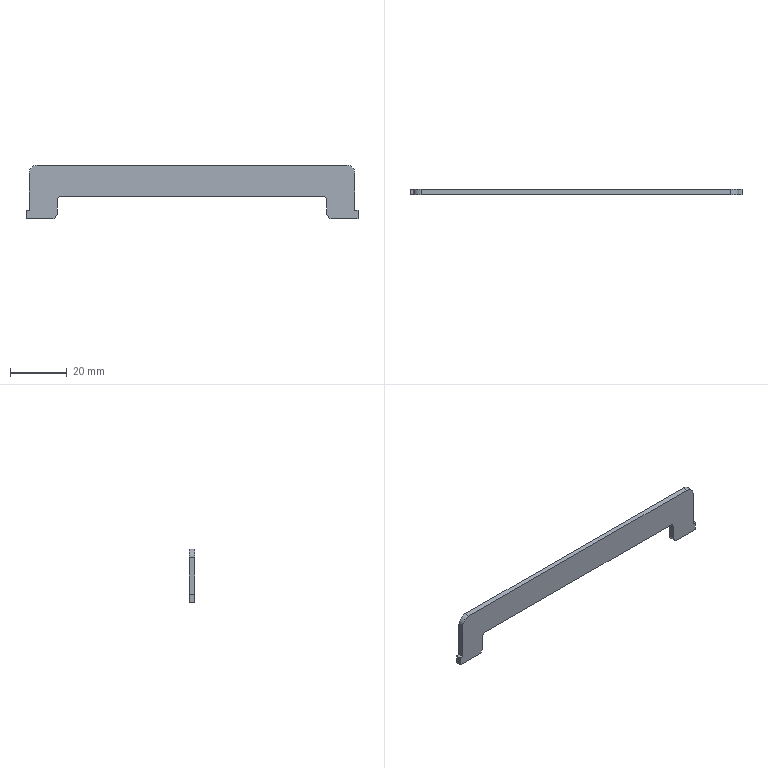Part | STEP file | 200 mesh_id2122 | 1 solid | 20 faces | box 117 x 1.9 x 19 mm | volume 2704 mm3 | plane 14 | cylinder 6 | commonest cylinder face diameters 3 x2 4 x2 6 x2
STEP:
#1=CARTESIAN_POINT('',(-16913.748,-3988.719,48.1));
#2=VERTEX_POINT('',#1);
#3=CARTESIAN_POINT('',(-17022.548,-3988.719,48.1));
#4=VERTEX_POINT('',#3);
#5=CARTESIAN_POINT('',(-16912.148,-3988.719,48.1));
#6=DIRECTION('',(-1.,0.,0.));
#7=VECTOR('',#6,1.);
#8=LINE('',#5,#7);
#9=EDGE_CURVE('',#2,#4,#8,.T.);
#10=ORIENTED_EDGE('',*,*,#9,.F.);
#11=CARTESIAN_POINT('',(-16913.748,-3986.819,48.1));
#12=VERTEX_POINT('',#11);
#13=CARTESIAN_POINT('',(-16913.748,-3988.744,48.1));
#14=DIRECTION('',(0.,1.,0.));
#15=VECTOR('',#14,1.);
#16=LINE('',#13,#15);
#17=EDGE_CURVE('',#2,#12,#16,.T.);
#18=ORIENTED_EDGE('',*,*,#17,.T.);
#19=CARTESIAN_POINT('',(-17022.548,-3986.819,48.1));
#20=VERTEX_POINT('',#19);
#21=CARTESIAN_POINT('',(-16912.148,-3986.819,48.1));
#22=DIRECTION('',(-1.,0.,0.));
#23=VECTOR('',#22,1.);
#24=LINE('',#21,#23);
#25=EDGE_CURVE('',#12,#20,#24,.T.);
#26=ORIENTED_EDGE('',*,*,#25,.T.);
#27=CARTESIAN_POINT('',(-17022.548,-3988.744,48.1));
#28=DIRECTION('',(0.,-1.,0.));
#29=VECTOR('',#28,1.);
#30=LINE('',#27,#29);
#31=EDGE_CURVE('',#20,#4,#30,.T.);
#32=ORIENTED_EDGE('',*,*,#31,.T.);
#33=EDGE_LOOP('',(#10,#18,#26,#32));
#34=FACE_OUTER_BOUND('',#33,.T.);
#35=CARTESIAN_POINT('',(-16912.148,-3988.744,48.1));
#36=DIRECTION('',(0.,0.,-1.));
#37=DIRECTION('',(1.,0.,0.));
#38=AXIS2_PLACEMENT_3D('',#35,#36,#37);
#39=PLANE('',#38);
#40=ADVANCED_FACE('',(#34),#39,.F.);
#41=CARTESIAN_POINT('',(-17025.548,-3988.719,45.1));
#42=VERTEX_POINT('',#41);
#43=CARTESIAN_POINT('',(-17025.548,-3988.719,32.1));
#44=VERTEX_POINT('',#43);
#45=CARTESIAN_POINT('',(-17025.548,-3988.719,46.6));
#46=DIRECTION('',(0.,0.,-1.));
#47=VECTOR('',#46,1.);
#48=LINE('',#45,#47);
#49=EDGE_CURVE('',#42,#44,#48,.T.);
#50=ORIENTED_EDGE('',*,*,#49,.F.);
#51=CARTESIAN_POINT('',(-17025.548,-3986.819,45.1));
#52=VERTEX_POINT('',#51);
#53=CARTESIAN_POINT('',(-17025.548,-3988.744,45.1));
#54=DIRECTION('',(0.,1.,0.));
#55=VECTOR('',#54,1.);
#56=LINE('',#53,#55);
#57=EDGE_CURVE('',#42,#52,#56,.T.);
#58=ORIENTED_EDGE('',*,*,#57,.T.);
#59=CARTESIAN_POINT('',(-17025.548,-3986.819,32.1));
#60=VERTEX_POINT('',#59);
#61=CARTESIAN_POINT('',(-17025.548,-3986.819,46.6));
#62=DIRECTION('',(0.,0.,-1.));
#63=VECTOR('',#62,1.);
#64=LINE('',#61,#63);
#65=EDGE_CURVE('',#52,#60,#64,.T.);
#66=ORIENTED_EDGE('',*,*,#65,.T.);
#67=CARTESIAN_POINT('',(-17025.548,-3988.744,32.1));
#68=DIRECTION('',(0.,1.,0.));
#69=VECTOR('',#68,1.);
#70=LINE('',#67,#69);
#71=EDGE_CURVE('',#44,#60,#70,.T.);
#72=ORIENTED_EDGE('',*,*,#71,.F.);
#73=EDGE_LOOP('',(#50,#58,#66,#72));
#74=FACE_OUTER_BOUND('',#73,.T.);
#75=CARTESIAN_POINT('',(-17025.548,-3988.744,46.6));
#76=DIRECTION('',(1.,0.,0.));
#77=DIRECTION('',(0.,1.,0.));
#78=AXIS2_PLACEMENT_3D('',#75,#76,#77);
#79=PLANE('',#78);
#80=ADVANCED_FACE('',(#74),#79,.F.);
#81=CARTESIAN_POINT('',(-17026.648,-3986.819,32.1));
#82=VERTEX_POINT('',#81);
#83=CARTESIAN_POINT('',(-17025.648,-3986.819,32.1));
#84=DIRECTION('',(-1.,0.,0.));
#85=VECTOR('',#84,1.);
#86=LINE('',#83,#85);
#87=EDGE_CURVE('',#60,#82,#86,.T.);
#88=ORIENTED_EDGE('',*,*,#87,.T.);
#89=CARTESIAN_POINT('',(-17026.648,-3988.719,32.1));
#90=VERTEX_POINT('',#89);
#91=CARTESIAN_POINT('',(-17026.648,-3988.744,32.1));
#92=DIRECTION('',(0.,1.,0.));
#93=VECTOR('',#92,1.);
#94=LINE('',#91,#93);
#95=EDGE_CURVE('',#90,#82,#94,.T.);
#96=ORIENTED_EDGE('',*,*,#95,.F.);
#97=CARTESIAN_POINT('',(-17025.648,-3988.719,32.1));
#98=DIRECTION('',(-1.,0.,0.));
#99=VECTOR('',#98,1.);
#100=LINE('',#97,#99);
#101=EDGE_CURVE('',#44,#90,#100,.T.);
#102=ORIENTED_EDGE('',*,*,#101,.F.);
#103=ORIENTED_EDGE('',*,*,#71,.T.);
#104=EDGE_LOOP('',(#88,#96,#102,#103));
#105=FACE_OUTER_BOUND('',#104,.T.);
#106=CARTESIAN_POINT('',(-17025.648,-3988.744,32.1));
#107=DIRECTION('',(0.,0.,-1.));
#108=DIRECTION('',(0.,1.,0.));
#109=AXIS2_PLACEMENT_3D('',#106,#107,#108);
#110=PLANE('',#109);
#111=ADVANCED_FACE('',(#105),#110,.F.);
#112=CARTESIAN_POINT('',(-17026.648,-3986.819,29.1));
#113=VERTEX_POINT('',#112);
#114=CARTESIAN_POINT('',(-17026.648,-3986.819,32.1));
#115=DIRECTION('',(0.,0.,-1.));
#116=VECTOR('',#115,1.);
#117=LINE('',#114,#116);
#118=EDGE_CURVE('',#82,#113,#117,.T.);
#119=ORIENTED_EDGE('',*,*,#118,.T.);
#120=CARTESIAN_POINT('',(-17026.648,-3988.719,29.1));
#121=VERTEX_POINT('',#120);
#122=CARTESIAN_POINT('',(-17026.648,-3988.744,29.1));
#123=DIRECTION('',(0.,1.,0.));
#124=VECTOR('',#123,1.);
#125=LINE('',#122,#124);
#126=EDGE_CURVE('',#121,#113,#125,.T.);
#127=ORIENTED_EDGE('',*,*,#126,.F.);
#128=CARTESIAN_POINT('',(-17026.648,-3988.719,32.1));
#129=DIRECTION('',(0.,0.,-1.));
#130=VECTOR('',#129,1.);
#131=LINE('',#128,#130);
#132=EDGE_CURVE('',#90,#121,#131,.T.);
#133=ORIENTED_EDGE('',*,*,#132,.F.);
#134=ORIENTED_EDGE('',*,*,#95,.T.);
#135=EDGE_LOOP('',(#119,#127,#133,#134));
#136=FACE_OUTER_BOUND('',#135,.T.);
#137=CARTESIAN_POINT('',(-17026.648,-3988.744,32.1));
#138=DIRECTION('',(1.,0.,0.));
#139=DIRECTION('',(0.,1.,0.));
#140=AXIS2_PLACEMENT_3D('',#137,#138,#139);
#141=PLANE('',#140);
#142=ADVANCED_FACE('',(#136),#141,.F.);
#143=CARTESIAN_POINT('',(-17017.648,-3986.819,29.1));
#144=VERTEX_POINT('',#143);
#145=CARTESIAN_POINT('',(-17026.648,-3986.819,29.1));
#146=DIRECTION('',(1.,0.,0.));
#147=VECTOR('',#146,1.);
#148=LINE('',#145,#147);
#149=EDGE_CURVE('',#113,#144,#148,.T.);
#150=ORIENTED_EDGE('',*,*,#149,.T.);
#151=CARTESIAN_POINT('',(-17017.648,-3988.719,29.1));
#152=VERTEX_POINT('',#151);
#153=CARTESIAN_POINT('',(-17017.648,-3988.744,29.1));
#154=DIRECTION('',(0.,-1.,0.));
#155=VECTOR('',#154,1.);
#156=LINE('',#153,#155);
#157=EDGE_CURVE('',#144,#152,#156,.T.);
#158=ORIENTED_EDGE('',*,*,#157,.T.);
#159=CARTESIAN_POINT('',(-17026.648,-3988.719,29.1));
#160=DIRECTION('',(1.,0.,0.));
#161=VECTOR('',#160,1.);
#162=LINE('',#159,#161);
#163=EDGE_CURVE('',#121,#152,#162,.T.);
#164=ORIENTED_EDGE('',*,*,#163,.F.);
#165=ORIENTED_EDGE('',*,*,#126,.T.);
#166=EDGE_LOOP('',(#150,#158,#164,#165));
#167=FACE_OUTER_BOUND('',#166,.T.);
#168=CARTESIAN_POINT('',(-17026.648,-3988.744,29.1));
#169=DIRECTION('',(0.,0.,1.));
#170=DIRECTION('',(0.,-1.,0.));
#171=AXIS2_PLACEMENT_3D('',#168,#169,#170);
#172=PLANE('',#171);
#173=ADVANCED_FACE('',(#167),#172,.F.);
#174=CARTESIAN_POINT('',(-17015.648,-3986.819,31.1));
#175=VERTEX_POINT('',#174);
#176=CARTESIAN_POINT('',(-17015.648,-3986.819,35.6));
#177=VERTEX_POINT('',#176);
#178=CARTESIAN_POINT('',(-17015.648,-3986.819,29.1));
#179=DIRECTION('',(0.,0.,1.));
#180=VECTOR('',#179,1.);
#181=LINE('',#178,#180);
#182=EDGE_CURVE('',#175,#177,#181,.T.);
#183=ORIENTED_EDGE('',*,*,#182,.T.);
#184=CARTESIAN_POINT('',(-17015.648,-3988.719,35.6));
#185=VERTEX_POINT('',#184);
#186=CARTESIAN_POINT('',(-17015.648,-3988.719,35.6));
#187=DIRECTION('',(0.,-1.,0.));
#188=VECTOR('',#187,1.);
#189=LINE('',#186,#188);
#190=EDGE_CURVE('',#177,#185,#189,.T.);
#191=ORIENTED_EDGE('',*,*,#190,.T.);
#192=CARTESIAN_POINT('',(-17015.648,-3988.719,31.1));
#193=VERTEX_POINT('',#192);
#194=CARTESIAN_POINT('',(-17015.648,-3988.719,29.1));
#195=DIRECTION('',(0.,0.,1.));
#196=VECTOR('',#195,1.);
#197=LINE('',#194,#196);
#198=EDGE_CURVE('',#193,#185,#197,.T.);
#199=ORIENTED_EDGE('',*,*,#198,.F.);
#200=CARTESIAN_POINT('',(-17015.648,-3988.744,31.1));
#201=DIRECTION('',(0.,1.,0.));
#202=VECTOR('',#201,1.);
#203=LINE('',#200,#202);
#204=EDGE_CURVE('',#193,#175,#203,.T.);
#205=ORIENTED_EDGE('',*,*,#204,.T.);
#206=EDGE_LOOP('',(#183,#191,#199,#205));
#207=FACE_OUTER_BOUND('',#206,.T.);
#208=CARTESIAN_POINT('',(-17015.648,-3988.744,29.1));
#209=DIRECTION('',(-1.,0.,0.));
#210=DIRECTION('',(0.,-1.,0.));
#211=AXIS2_PLACEMENT_3D('',#208,#209,#210);
#212=PLANE('',#211);
#213=ADVANCED_FACE('',(#207),#212,.F.);
#214=CARTESIAN_POINT('',(-17014.148,-3988.719,37.1));
#215=VERTEX_POINT('',#214);
#216=CARTESIAN_POINT('',(-16922.148,-3988.719,37.1));
#217=VERTEX_POINT('',#216);
#218=CARTESIAN_POINT('',(-17015.648,-3988.719,37.1));
#219=DIRECTION('',(1.,0.,0.));
#220=VECTOR('',#219,1.);
#221=LINE('',#218,#220);
#222=EDGE_CURVE('',#215,#217,#221,.T.);
#223=ORIENTED_EDGE('',*,*,#222,.F.);
#224=CARTESIAN_POINT('',(-17014.148,-3986.819,37.1));
#225=VERTEX_POINT('',#224);
#226=CARTESIAN_POINT('',(-17014.148,-3986.819,37.1));
#227=DIRECTION('',(0.,1.,0.));
#228=VECTOR('',#227,1.);
#229=LINE('',#226,#228);
#230=EDGE_CURVE('',#215,#225,#229,.T.);
#231=ORIENTED_EDGE('',*,*,#230,.T.);
#232=CARTESIAN_POINT('',(-16922.148,-3986.819,37.1));
#233=VERTEX_POINT('',#232);
#234=CARTESIAN_POINT('',(-17015.648,-3986.819,37.1));
#235=DIRECTION('',(1.,0.,0.));
#236=VECTOR('',#235,1.);
#237=LINE('',#234,#236);
#238=EDGE_CURVE('',#225,#233,#237,.T.);
#239=ORIENTED_EDGE('',*,*,#238,.T.);
#240=CARTESIAN_POINT('',(-16922.148,-3988.719,37.1));
#241=DIRECTION('',(0.,-1.,0.));
#242=VECTOR('',#241,1.);
#243=LINE('',#240,#242);
#244=EDGE_CURVE('',#233,#217,#243,.T.);
#245=ORIENTED_EDGE('',*,*,#244,.T.);
#246=EDGE_LOOP('',(#223,#231,#239,#245));
#247=FACE_OUTER_BOUND('',#246,.T.);
#248=CARTESIAN_POINT('',(-17015.648,-3988.744,37.1));
#249=DIRECTION('',(0.,0.,1.));
#250=DIRECTION('',(0.,-1.,0.));
#251=AXIS2_PLACEMENT_3D('',#248,#249,#250);
#252=PLANE('',#251);
#253=ADVANCED_FACE('',(#247),#252,.F.);
#254=CARTESIAN_POINT('',(-16920.648,-3988.719,35.6));
#255=VERTEX_POINT('',#254);
#256=CARTESIAN_POINT('',(-16920.648,-3988.719,31.1));
#257=VERTEX_POINT('',#256);
#258=CARTESIAN_POINT('',(-16920.648,-3988.719,37.1));
#259=DIRECTION('',(0.,0.,-1.));
#260=VECTOR('',#259,1.);
#261=LINE('',#258,#260);
#262=EDGE_CURVE('',#255,#257,#261,.T.);
#263=ORIENTED_EDGE('',*,*,#262,.F.);
#264=CARTESIAN_POINT('',(-16920.648,-3986.819,35.6));
#265=VERTEX_POINT('',#264);
#266=CARTESIAN_POINT('',(-16920.648,-3986.819,35.6));
#267=DIRECTION('',(0.,1.,0.));
#268=VECTOR('',#267,1.);
#269=LINE('',#266,#268);
#270=EDGE_CURVE('',#255,#265,#269,.T.);
#271=ORIENTED_EDGE('',*,*,#270,.T.);
#272=CARTESIAN_POINT('',(-16920.648,-3986.819,31.1));
#273=VERTEX_POINT('',#272);
#274=CARTESIAN_POINT('',(-16920.648,-3986.819,37.1));
#275=DIRECTION('',(0.,0.,-1.));
#276=VECTOR('',#275,1.);
#277=LINE('',#274,#276);
#278=EDGE_CURVE('',#265,#273,#277,.T.);
#279=ORIENTED_EDGE('',*,*,#278,.T.);
#280=CARTESIAN_POINT('',(-16920.648,-3988.744,31.1));
#281=DIRECTION('',(0.,-1.,0.));
#282=VECTOR('',#281,1.);
#283=LINE('',#280,#282);
#284=EDGE_CURVE('',#273,#257,#283,.T.);
#285=ORIENTED_EDGE('',*,*,#284,.T.);
#286=EDGE_LOOP('',(#263,#271,#279,#285));
#287=FACE_OUTER_BOUND('',#286,.T.);
#288=CARTESIAN_POINT('',(-16920.648,-3988.744,37.1));
#289=DIRECTION('',(1.,0.,0.));
#290=DIRECTION('',(0.,1.,0.));
#291=AXIS2_PLACEMENT_3D('',#288,#289,#290);
#292=PLANE('',#291);
#293=ADVANCED_FACE('',(#287),#292,.F.);
#294=CARTESIAN_POINT('',(-16918.648,-3988.719,29.1));
#295=VERTEX_POINT('',#294);
#296=CARTESIAN_POINT('',(-16909.648,-3988.719,29.1));
#297=VERTEX_POINT('',#296);
#298=CARTESIAN_POINT('',(-16920.648,-3988.719,29.1));
#299=DIRECTION('',(1.,0.,0.));
#300=VECTOR('',#299,1.);
#301=LINE('',#298,#300);
#302=EDGE_CURVE('',#295,#297,#301,.T.);
#303=ORIENTED_EDGE('',*,*,#302,.F.);
#304=CARTESIAN_POINT('',(-16918.648,-3986.819,29.1));
#305=VERTEX_POINT('',#304);
#306=CARTESIAN_POINT('',(-16918.648,-3988.744,29.1));
#307=DIRECTION('',(0.,1.,0.));
#308=VECTOR('',#307,1.);
#309=LINE('',#306,#308);
#310=EDGE_CURVE('',#295,#305,#309,.T.);
#311=ORIENTED_EDGE('',*,*,#310,.T.);
#312=CARTESIAN_POINT('',(-16909.648,-3986.819,29.1));
#313=VERTEX_POINT('',#312);
#314=CARTESIAN_POINT('',(-16920.648,-3986.819,29.1));
#315=DIRECTION('',(1.,0.,0.));
#316=VECTOR('',#315,1.);
#317=LINE('',#314,#316);
#318=EDGE_CURVE('',#305,#313,#317,.T.);
#319=ORIENTED_EDGE('',*,*,#318,.T.);
#320=CARTESIAN_POINT('',(-16909.648,-3988.744,29.1));
#321=DIRECTION('',(0.,1.,0.));
#322=VECTOR('',#321,1.);
#323=LINE('',#320,#322);
#324=EDGE_CURVE('',#297,#313,#323,.T.);
#325=ORIENTED_EDGE('',*,*,#324,.F.);
#326=EDGE_LOOP('',(#303,#311,#319,#325));
#327=FACE_OUTER_BOUND('',#326,.T.);
#328=CARTESIAN_POINT('',(-16920.648,-3988.744,29.1));
#329=DIRECTION('',(0.,0.,1.));
#330=DIRECTION('',(0.,-1.,0.));
#331=AXIS2_PLACEMENT_3D('',#328,#329,#330);
#332=PLANE('',#331);
#333=ADVANCED_FACE('',(#327),#332,.F.);
#334=CARTESIAN_POINT('',(-16909.648,-3986.819,32.1));
#335=VERTEX_POINT('',#334);
#336=CARTESIAN_POINT('',(-16909.648,-3986.819,29.1));
#337=DIRECTION('',(0.,0.,1.));
#338=VECTOR('',#337,1.);
#339=LINE('',#336,#338);
#340=EDGE_CURVE('',#313,#335,#339,.T.);
#341=ORIENTED_EDGE('',*,*,#340,.T.);
#342=CARTESIAN_POINT('',(-16909.648,-3988.719,32.1));
#343=VERTEX_POINT('',#342);
#344=CARTESIAN_POINT('',(-16909.648,-3988.744,32.1));
#345=DIRECTION('',(0.,1.,0.));
#346=VECTOR('',#345,1.);
#347=LINE('',#344,#346);
#348=EDGE_CURVE('',#343,#335,#347,.T.);
#349=ORIENTED_EDGE('',*,*,#348,.F.);
#350=CARTESIAN_POINT('',(-16909.648,-3988.719,29.1));
#351=DIRECTION('',(0.,0.,1.));
#352=VECTOR('',#351,1.);
#353=LINE('',#350,#352);
#354=EDGE_CURVE('',#297,#343,#353,.T.);
#355=ORIENTED_EDGE('',*,*,#354,.F.);
#356=ORIENTED_EDGE('',*,*,#324,.T.);
#357=EDGE_LOOP('',(#341,#349,#355,#356));
#358=FACE_OUTER_BOUND('',#357,.T.);
#359=CARTESIAN_POINT('',(-16909.648,-3988.744,29.1));
#360=DIRECTION('',(-1.,0.,0.));
#361=DIRECTION('',(0.,-1.,0.));
#362=AXIS2_PLACEMENT_3D('',#359,#360,#361);
#363=PLANE('',#362);
#364=ADVANCED_FACE('',(#358),#363,.F.);
#365=CARTESIAN_POINT('',(-16910.748,-3986.819,32.1));
#366=VERTEX_POINT('',#365);
#367=CARTESIAN_POINT('',(-16909.648,-3986.819,32.1));
#368=DIRECTION('',(-1.,0.,0.));
#369=VECTOR('',#368,1.);
#370=LINE('',#367,#369);
#371=EDGE_CURVE('',#335,#366,#370,.T.);
#372=ORIENTED_EDGE('',*,*,#371,.T.);
#373=CARTESIAN_POINT('',(-16910.748,-3988.719,32.1));
#374=VERTEX_POINT('',#373);
#375=CARTESIAN_POINT('',(-16910.748,-3988.744,32.1));
#376=DIRECTION('',(0.,1.,0.));
#377=VECTOR('',#376,1.);
#378=LINE('',#375,#377);
#379=EDGE_CURVE('',#374,#366,#378,.T.);
#380=ORIENTED_EDGE('',*,*,#379,.F.);
#381=CARTESIAN_POINT('',(-16909.648,-3988.719,32.1));
#382=DIRECTION('',(-1.,0.,0.));
#383=VECTOR('',#382,1.);
#384=LINE('',#381,#383);
#385=EDGE_CURVE('',#343,#374,#384,.T.);
#386=ORIENTED_EDGE('',*,*,#385,.F.);
#387=ORIENTED_EDGE('',*,*,#348,.T.);
#388=EDGE_LOOP('',(#372,#380,#386,#387));
#389=FACE_OUTER_BOUND('',#388,.T.);
#390=CARTESIAN_POINT('',(-16909.648,-3988.744,32.1));
#391=DIRECTION('',(0.,0.,-1.));
#392=DIRECTION('',(0.,1.,0.));
#393=AXIS2_PLACEMENT_3D('',#390,#391,#392);
#394=PLANE('',#393);
#395=ADVANCED_FACE('',(#389),#394,.F.);
#396=CARTESIAN_POINT('',(-16910.748,-3986.819,45.1));
#397=VERTEX_POINT('',#396);
#398=CARTESIAN_POINT('',(-16910.748,-3986.819,32.1));
#399=DIRECTION('',(0.,0.,1.));
#400=VECTOR('',#399,1.);
#401=LINE('',#398,#400);
#402=EDGE_CURVE('',#366,#397,#401,.T.);
#403=ORIENTED_EDGE('',*,*,#402,.T.);
#404=CARTESIAN_POINT('',(-16910.748,-3988.719,45.1));
#405=VERTEX_POINT('',#404);
#406=CARTESIAN_POINT('',(-16910.748,-3988.744,45.1));
#407=DIRECTION('',(0.,-1.,0.));
#408=VECTOR('',#407,1.);
#409=LINE('',#406,#408);
#410=EDGE_CURVE('',#397,#405,#409,.T.);
#411=ORIENTED_EDGE('',*,*,#410,.T.);
#412=CARTESIAN_POINT('',(-16910.748,-3988.719,32.1));
#413=DIRECTION('',(0.,0.,1.));
#414=VECTOR('',#413,1.);
#415=LINE('',#412,#414);
#416=EDGE_CURVE('',#374,#405,#415,.T.);
#417=ORIENTED_EDGE('',*,*,#416,.F.);
#418=ORIENTED_EDGE('',*,*,#379,.T.);
#419=EDGE_LOOP('',(#403,#411,#417,#418));
#420=FACE_OUTER_BOUND('',#419,.T.);
#421=CARTESIAN_POINT('',(-16910.748,-3988.744,32.1));
#422=DIRECTION('',(-1.,0.,0.));
#423=DIRECTION('',(0.,-1.,0.));
#424=AXIS2_PLACEMENT_3D('',#421,#422,#423);
#425=PLANE('',#424);
#426=ADVANCED_FACE('',(#420),#425,.F.);
#427=ORIENTED_EDGE('',*,*,#198,.T.);
#428=CARTESIAN_POINT('',(-17014.148,-3988.719,35.6));
#429=DIRECTION('',(0.,1.,0.));
#430=DIRECTION('',(0.,0.,-1.));
#431=AXIS2_PLACEMENT_3D('',#428,#429,#430);
#432=CIRCLE('',#431,1.5);
#433=EDGE_CURVE('',#185,#215,#432,.T.);
#434=ORIENTED_EDGE('',*,*,#433,.T.);
#435=ORIENTED_EDGE('',*,*,#222,.T.);
#436=CARTESIAN_POINT('',(-16922.148,-3988.719,35.6));
#437=DIRECTION('',(0.,1.,0.));
#438=DIRECTION('',(0.,0.,-1.));
#439=AXIS2_PLACEMENT_3D('',#436,#437,#438);
#440=CIRCLE('',#439,1.5);
#441=EDGE_CURVE('',#217,#255,#440,.T.);
#442=ORIENTED_EDGE('',*,*,#441,.T.);
#443=ORIENTED_EDGE('',*,*,#262,.T.);
#444=CARTESIAN_POINT('',(-16918.648,-3988.719,31.1));
#445=DIRECTION('',(0.,-1.,0.));
#446=DIRECTION('',(0.,0.,-1.));
#447=AXIS2_PLACEMENT_3D('',#444,#445,#446);
#448=CIRCLE('',#447,2.);
#449=EDGE_CURVE('',#257,#295,#448,.T.);
#450=ORIENTED_EDGE('',*,*,#449,.T.);
#451=ORIENTED_EDGE('',*,*,#302,.T.);
#452=ORIENTED_EDGE('',*,*,#354,.T.);
#453=ORIENTED_EDGE('',*,*,#385,.T.);
#454=ORIENTED_EDGE('',*,*,#416,.T.);
#455=CARTESIAN_POINT('',(-16913.748,-3988.719,45.1));
#456=DIRECTION('',(0.,-1.,0.));
#457=DIRECTION('',(0.,0.,-1.));
#458=AXIS2_PLACEMENT_3D('',#455,#456,#457);
#459=CIRCLE('',#458,3.);
#460=EDGE_CURVE('',#405,#2,#459,.T.);
#461=ORIENTED_EDGE('',*,*,#460,.T.);
#462=ORIENTED_EDGE('',*,*,#9,.T.);
#463=CARTESIAN_POINT('',(-17022.548,-3988.719,45.1));
#464=DIRECTION('',(0.,-1.,0.));
#465=DIRECTION('',(0.,0.,-1.));
#466=AXIS2_PLACEMENT_3D('',#463,#464,#465);
#467=CIRCLE('',#466,3.);
#468=EDGE_CURVE('',#4,#42,#467,.T.);
#469=ORIENTED_EDGE('',*,*,#468,.T.);
#470=ORIENTED_EDGE('',*,*,#49,.T.);
#471=ORIENTED_EDGE('',*,*,#101,.T.);
#472=ORIENTED_EDGE('',*,*,#132,.T.);
#473=ORIENTED_EDGE('',*,*,#163,.T.);
#474=CARTESIAN_POINT('',(-17017.648,-3988.719,31.1));
#475=DIRECTION('',(0.,-1.,0.));
#476=DIRECTION('',(0.,0.,-1.));
#477=AXIS2_PLACEMENT_3D('',#474,#475,#476);
#478=CIRCLE('',#477,2.);
#479=EDGE_CURVE('',#152,#193,#478,.T.);
#480=ORIENTED_EDGE('',*,*,#479,.T.);
#481=EDGE_LOOP('',(#427,#434,#435,#442,#443,#450,#451,#452,#453,#454,#461,#462,#469,#470,#471,#472,#473,#480));
#482=FACE_OUTER_BOUND('',#481,.T.);
#483=CARTESIAN_POINT('',(-17024.148,-3988.719,46.6));
#484=DIRECTION('',(0.,-1.,0.));
#485=DIRECTION('',(1.,0.,0.));
#486=AXIS2_PLACEMENT_3D('',#483,#484,#485);
#487=PLANE('',#486);
#488=ADVANCED_FACE('',(#482),#487,.T.);
#489=ORIENTED_EDGE('',*,*,#318,.F.);
#490=CARTESIAN_POINT('',(-16918.648,-3986.819,31.1));
#491=DIRECTION('',(0.,1.,0.));
#492=DIRECTION('',(0.,0.,-1.));
#493=AXIS2_PLACEMENT_3D('',#490,#491,#492);
#494=CIRCLE('',#493,2.);
#495=EDGE_CURVE('',#305,#273,#494,.T.);
#496=ORIENTED_EDGE('',*,*,#495,.T.);
#497=ORIENTED_EDGE('',*,*,#278,.F.);
#498=CARTESIAN_POINT('',(-16922.148,-3986.819,35.6));
#499=DIRECTION('',(0.,-1.,0.));
#500=DIRECTION('',(0.,0.,-1.));
#501=AXIS2_PLACEMENT_3D('',#498,#499,#500);
#502=CIRCLE('',#501,1.5);
#503=EDGE_CURVE('',#265,#233,#502,.T.);
#504=ORIENTED_EDGE('',*,*,#503,.T.);
#505=ORIENTED_EDGE('',*,*,#238,.F.);
#506=CARTESIAN_POINT('',(-17014.148,-3986.819,35.6));
#507=DIRECTION('',(0.,-1.,0.));
#508=DIRECTION('',(0.,0.,-1.));
#509=AXIS2_PLACEMENT_3D('',#506,#507,#508);
#510=CIRCLE('',#509,1.5);
#511=EDGE_CURVE('',#225,#177,#510,.T.);
#512=ORIENTED_EDGE('',*,*,#511,.T.);
#513=ORIENTED_EDGE('',*,*,#182,.F.);
#514=CARTESIAN_POINT('',(-17017.648,-3986.819,31.1));
#515=DIRECTION('',(0.,1.,0.));
#516=DIRECTION('',(0.,0.,-1.));
#517=AXIS2_PLACEMENT_3D('',#514,#515,#516);
#518=CIRCLE('',#517,2.);
#519=EDGE_CURVE('',#175,#144,#518,.T.);
#520=ORIENTED_EDGE('',*,*,#519,.T.);
#521=ORIENTED_EDGE('',*,*,#149,.F.);
#522=ORIENTED_EDGE('',*,*,#118,.F.);
#523=ORIENTED_EDGE('',*,*,#87,.F.);
#524=ORIENTED_EDGE('',*,*,#65,.F.);
#525=CARTESIAN_POINT('',(-17022.548,-3986.819,45.1));
#526=DIRECTION('',(0.,1.,0.));
#527=DIRECTION('',(0.,0.,-1.));
#528=AXIS2_PLACEMENT_3D('',#525,#526,#527);
#529=CIRCLE('',#528,3.);
#530=EDGE_CURVE('',#52,#20,#529,.T.);
#531=ORIENTED_EDGE('',*,*,#530,.T.);
#532=ORIENTED_EDGE('',*,*,#25,.F.);
#533=CARTESIAN_POINT('',(-16913.748,-3986.819,45.1));
#534=DIRECTION('',(0.,1.,0.));
#535=DIRECTION('',(0.,0.,-1.));
#536=AXIS2_PLACEMENT_3D('',#533,#534,#535);
#537=CIRCLE('',#536,3.);
#538=EDGE_CURVE('',#12,#397,#537,.T.);
#539=ORIENTED_EDGE('',*,*,#538,.T.);
#540=ORIENTED_EDGE('',*,*,#402,.F.);
#541=ORIENTED_EDGE('',*,*,#371,.F.);
#542=ORIENTED_EDGE('',*,*,#340,.F.);
#543=EDGE_LOOP('',(#489,#496,#497,#504,#505,#512,#513,#520,#521,#522,#523,#524,#531,#532,#539,#540,#541,#542));
#544=FACE_OUTER_BOUND('',#543,.T.);
#545=CARTESIAN_POINT('',(-17024.148,-3986.819,46.6));
#546=DIRECTION('',(0.,-1.,0.));
#547=DIRECTION('',(1.,0.,0.));
#548=AXIS2_PLACEMENT_3D('',#545,#546,#547);
#549=PLANE('',#548);
#550=ADVANCED_FACE('',(#544),#549,.F.);
#551=ORIENTED_EDGE('',*,*,#460,.F.);
#552=ORIENTED_EDGE('',*,*,#410,.F.);
#553=ORIENTED_EDGE('',*,*,#538,.F.);
#554=ORIENTED_EDGE('',*,*,#17,.F.);
#555=EDGE_LOOP('',(#551,#552,#553,#554));
#556=FACE_OUTER_BOUND('',#555,.T.);
#557=CARTESIAN_POINT('',(-16913.748,-3988.744,45.1));
#558=DIRECTION('',(0.,1.,0.));
#559=DIRECTION('',(0.,0.,1.));
#560=AXIS2_PLACEMENT_3D('',#557,#558,#559);
#561=CYLINDRICAL_SURFACE('',#560,3.);
#562=ADVANCED_FACE('',(#556),#561,.T.);
#563=ORIENTED_EDGE('',*,*,#468,.F.);
#564=ORIENTED_EDGE('',*,*,#31,.F.);
#565=ORIENTED_EDGE('',*,*,#530,.F.);
#566=ORIENTED_EDGE('',*,*,#57,.F.);
#567=EDGE_LOOP('',(#563,#564,#565,#566));
#568=FACE_OUTER_BOUND('',#567,.T.);
#569=CARTESIAN_POINT('',(-17022.548,-3988.744,45.1));
#570=DIRECTION('',(0.,1.,0.));
#571=DIRECTION('',(0.,0.,1.));
#572=AXIS2_PLACEMENT_3D('',#569,#570,#571);
#573=CYLINDRICAL_SURFACE('',#572,3.);
#574=ADVANCED_FACE('',(#568),#573,.T.);
#575=ORIENTED_EDGE('',*,*,#479,.F.);
#576=ORIENTED_EDGE('',*,*,#157,.F.);
#577=ORIENTED_EDGE('',*,*,#519,.F.);
#578=ORIENTED_EDGE('',*,*,#204,.F.);
#579=EDGE_LOOP('',(#575,#576,#577,#578));
#580=FACE_OUTER_BOUND('',#579,.T.);
#581=CARTESIAN_POINT('',(-17017.648,-3988.744,31.1));
#582=DIRECTION('',(0.,1.,0.));
#583=DIRECTION('',(0.,0.,1.));
#584=AXIS2_PLACEMENT_3D('',#581,#582,#583);
#585=CYLINDRICAL_SURFACE('',#584,2.);
#586=ADVANCED_FACE('',(#580),#585,.T.);
#587=ORIENTED_EDGE('',*,*,#449,.F.);
#588=ORIENTED_EDGE('',*,*,#284,.F.);
#589=ORIENTED_EDGE('',*,*,#495,.F.);
#590=ORIENTED_EDGE('',*,*,#310,.F.);
#591=EDGE_LOOP('',(#587,#588,#589,#590));
#592=FACE_OUTER_BOUND('',#591,.T.);
#593=CARTESIAN_POINT('',(-16918.648,-3988.744,31.1));
#594=DIRECTION('',(0.,1.,0.));
#595=DIRECTION('',(0.,0.,1.));
#596=AXIS2_PLACEMENT_3D('',#593,#594,#595);
#597=CYLINDRICAL_SURFACE('',#596,2.);
#598=ADVANCED_FACE('',(#592),#597,.T.);
#599=ORIENTED_EDGE('',*,*,#441,.F.);
#600=ORIENTED_EDGE('',*,*,#244,.F.);
#601=ORIENTED_EDGE('',*,*,#503,.F.);
#602=ORIENTED_EDGE('',*,*,#270,.F.);
#603=EDGE_LOOP('',(#599,#600,#601,#602));
#604=FACE_OUTER_BOUND('',#603,.T.);
#605=CARTESIAN_POINT('',(-16922.148,-3988.744,35.6));
#606=DIRECTION('',(0.,-1.,0.));
#607=DIRECTION('',(0.,0.,-1.));
#608=AXIS2_PLACEMENT_3D('',#605,#606,#607);
#609=CYLINDRICAL_SURFACE('',#608,1.5);
#610=ADVANCED_FACE('',(#604),#609,.F.);
#611=ORIENTED_EDGE('',*,*,#433,.F.);
#612=ORIENTED_EDGE('',*,*,#190,.F.);
#613=ORIENTED_EDGE('',*,*,#511,.F.);
#614=ORIENTED_EDGE('',*,*,#230,.F.);
#615=EDGE_LOOP('',(#611,#612,#613,#614));
#616=FACE_OUTER_BOUND('',#615,.T.);
#617=CARTESIAN_POINT('',(-17014.148,-3988.744,35.6));
#618=DIRECTION('',(0.,-1.,0.));
#619=DIRECTION('',(0.,0.,-1.));
#620=AXIS2_PLACEMENT_3D('',#617,#618,#619);
#621=CYLINDRICAL_SURFACE('',#620,1.5);
#622=ADVANCED_FACE('',(#616),#621,.F.);
#623=CLOSED_SHELL('',(#40,#80,#111,#142,#173,#213,#253,#293,#333,#364,#395,#426,#488,#550,#562,#574,#586,#598,#610,#622));
#624=MANIFOLD_SOLID_BREP('',#623);
#625=(LENGTH_UNIT()NAMED_UNIT(*)SI_UNIT(.MILLI.,.METRE.));
#626=UNCERTAINTY_MEASURE_WITH_UNIT(LENGTH_MEASURE(0.00002),#625,'','');
#627=(NAMED_UNIT(*)PLANE_ANGLE_UNIT()SI_UNIT($,.RADIAN.));
#628=PLANE_ANGLE_MEASURE_WITH_UNIT(PLANE_ANGLE_MEASURE(0.01745),#627);
#629=DIMENSIONAL_EXPONENTS(0.,0.,0.,0.,0.,0.,0.);
#630=(CONVERSION_BASED_UNIT('DEGREE',#628)NAMED_UNIT(#629)PLANE_ANGLE_UNIT());
#631=(NAMED_UNIT(*)SI_UNIT($,.STERADIAN.)SOLID_ANGLE_UNIT());
#632=(GEOMETRIC_REPRESENTATION_CONTEXT(3)GLOBAL_UNCERTAINTY_ASSIGNED_CONTEXT((#626))GLOBAL_UNIT_ASSIGNED_CONTEXT((#625,#630,#631))REPRESENTATION_CONTEXT('',''));
#633=ADVANCED_BREP_SHAPE_REPRESENTATION('',(#624),#632);